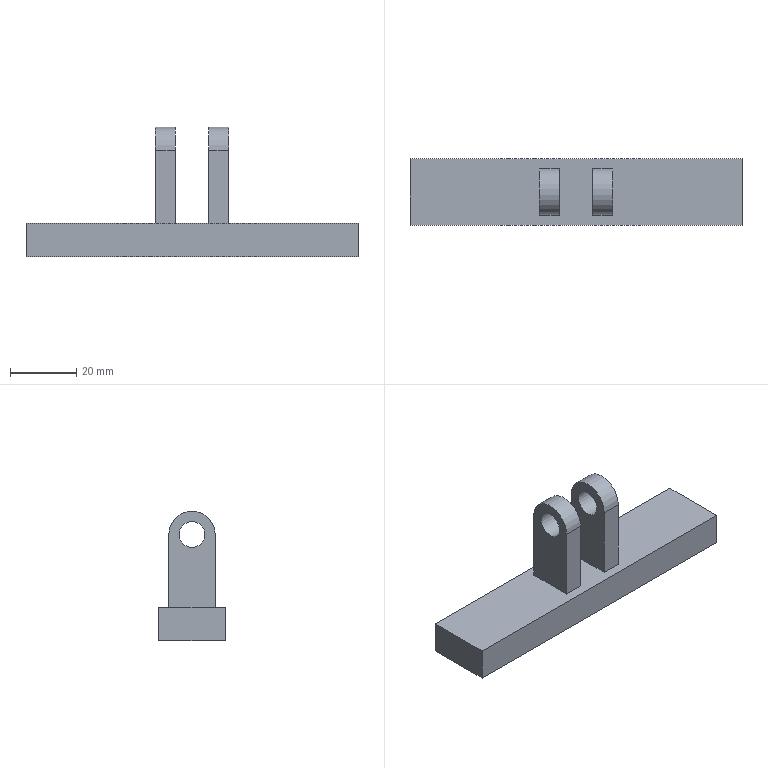Part | NX | features DATUM_CSYS 2, BLEND 1, BLOCK 1, EXTRUDE 1, HOLE PACKAGE 1, SIMPLE HOLE 1, SKETCH 1 | 1 solid | 18 faces | box 100 x 20 x 39 mm | volume 24046 mm3 | plane 14 | cylinder 4 | commonest cylinder face diameters 7.8 x2 14 x2
STEP:
#1=CARTESIAN_POINT('',(-11.,7.,10.));
#2=VERTEX_POINT('',#1);
#3=CARTESIAN_POINT('',(-11.,-7.,10.));
#4=VERTEX_POINT('',#3);
#5=CARTESIAN_POINT('',(-11.,7.,10.));
#6=DIRECTION('',(0.,-1.,0.));
#7=VECTOR('',#6,1000.);
#8=LINE('',#5,#7);
#9=EDGE_CURVE('',#2,#4,#8,.T.);
#10=ORIENTED_EDGE('',*,*,#9,.F.);
#11=CARTESIAN_POINT('',(-5.,7.,10.));
#12=VERTEX_POINT('',#11);
#13=CARTESIAN_POINT('',(-5.,7.,10.));
#14=DIRECTION('',(-1.,0.,0.));
#15=VECTOR('',#14,1000.);
#16=LINE('',#13,#15);
#17=EDGE_CURVE('',#12,#2,#16,.T.);
#18=ORIENTED_EDGE('',*,*,#17,.F.);
#19=CARTESIAN_POINT('',(-5.,-7.,10.));
#20=VERTEX_POINT('',#19);
#21=CARTESIAN_POINT('',(-5.,-7.,10.));
#22=DIRECTION('',(0.,1.,0.));
#23=VECTOR('',#22,1000.);
#24=LINE('',#21,#23);
#25=EDGE_CURVE('',#20,#12,#24,.T.);
#26=ORIENTED_EDGE('',*,*,#25,.F.);
#27=CARTESIAN_POINT('',(-11.,-7.,10.));
#28=DIRECTION('',(1.,0.,0.));
#29=VECTOR('',#28,1000.);
#30=LINE('',#27,#29);
#31=EDGE_CURVE('',#4,#20,#30,.T.);
#32=ORIENTED_EDGE('',*,*,#31,.F.);
#33=EDGE_LOOP('',(#10,#18,#26,#32));
#34=FACE_BOUND('',#33,.T.);
#35=CARTESIAN_POINT('',(5.,7.,10.));
#36=VERTEX_POINT('',#35);
#37=CARTESIAN_POINT('',(5.,-7.,10.));
#38=VERTEX_POINT('',#37);
#39=CARTESIAN_POINT('',(5.,7.,10.));
#40=DIRECTION('',(0.,-1.,0.));
#41=VECTOR('',#40,1000.);
#42=LINE('',#39,#41);
#43=EDGE_CURVE('',#36,#38,#42,.T.);
#44=ORIENTED_EDGE('',*,*,#43,.F.);
#45=CARTESIAN_POINT('',(11.,7.,10.));
#46=VERTEX_POINT('',#45);
#47=CARTESIAN_POINT('',(11.,7.,10.));
#48=DIRECTION('',(-1.,0.,0.));
#49=VECTOR('',#48,1000.);
#50=LINE('',#47,#49);
#51=EDGE_CURVE('',#46,#36,#50,.T.);
#52=ORIENTED_EDGE('',*,*,#51,.F.);
#53=CARTESIAN_POINT('',(11.,-7.,10.));
#54=VERTEX_POINT('',#53);
#55=CARTESIAN_POINT('',(11.,-7.,10.));
#56=DIRECTION('',(0.,1.,0.));
#57=VECTOR('',#56,1000.);
#58=LINE('',#55,#57);
#59=EDGE_CURVE('',#54,#46,#58,.T.);
#60=ORIENTED_EDGE('',*,*,#59,.F.);
#61=CARTESIAN_POINT('',(5.,-7.,10.));
#62=DIRECTION('',(1.,0.,0.));
#63=VECTOR('',#62,1000.);
#64=LINE('',#61,#63);
#65=EDGE_CURVE('',#38,#54,#64,.T.);
#66=ORIENTED_EDGE('',*,*,#65,.F.);
#67=EDGE_LOOP('',(#44,#52,#60,#66));
#68=FACE_BOUND('',#67,.T.);
#69=CARTESIAN_POINT('',(50.,-10.,10.));
#70=VERTEX_POINT('',#69);
#71=CARTESIAN_POINT('',(-50.,-10.,10.));
#72=VERTEX_POINT('',#71);
#73=CARTESIAN_POINT('',(0.,-10.,10.));
#74=DIRECTION('',(-1.,0.,0.));
#75=VECTOR('',#74,1000.);
#76=LINE('',#73,#75);
#77=EDGE_CURVE('',#70,#72,#76,.T.);
#78=ORIENTED_EDGE('',*,*,#77,.F.);
#79=CARTESIAN_POINT('',(50.,10.,10.));
#80=VERTEX_POINT('',#79);
#81=CARTESIAN_POINT('',(50.,0.,10.));
#82=DIRECTION('',(0.,-1.,0.));
#83=VECTOR('',#82,1000.);
#84=LINE('',#81,#83);
#85=EDGE_CURVE('',#80,#70,#84,.T.);
#86=ORIENTED_EDGE('',*,*,#85,.F.);
#87=CARTESIAN_POINT('',(-50.,10.,10.));
#88=VERTEX_POINT('',#87);
#89=CARTESIAN_POINT('',(0.,10.,10.));
#90=DIRECTION('',(1.,0.,0.));
#91=VECTOR('',#90,1000.);
#92=LINE('',#89,#91);
#93=EDGE_CURVE('',#88,#80,#92,.T.);
#94=ORIENTED_EDGE('',*,*,#93,.F.);
#95=CARTESIAN_POINT('',(-50.,0.,10.));
#96=DIRECTION('',(0.,1.,0.));
#97=VECTOR('',#96,1000.);
#98=LINE('',#95,#97);
#99=EDGE_CURVE('',#72,#88,#98,.T.);
#100=ORIENTED_EDGE('',*,*,#99,.F.);
#101=EDGE_LOOP('',(#78,#86,#94,#100));
#102=FACE_BOUND('',#101,.T.);
#103=CARTESIAN_POINT('',(0.,0.,10.));
#104=DIRECTION('',(0.,0.,1.));
#105=DIRECTION('',(1.,0.,0.));
#106=AXIS2_PLACEMENT_3D('',#103,#104,#105);
#107=PLANE('',#106);
#108=ADVANCED_FACE('',(#34,#68,#102),#107,.T.);
#109=CARTESIAN_POINT('',(50.,-10.,0.));
#110=VERTEX_POINT('',#109);
#111=CARTESIAN_POINT('',(50.,-10.,0.));
#112=DIRECTION('',(0.,0.,1.));
#113=VECTOR('',#112,1000.);
#114=LINE('',#111,#113);
#115=EDGE_CURVE('',#110,#70,#114,.T.);
#116=ORIENTED_EDGE('',*,*,#115,.T.);
#117=ORIENTED_EDGE('',*,*,#77,.T.);
#118=CARTESIAN_POINT('',(-50.,-10.,0.));
#119=VERTEX_POINT('',#118);
#120=CARTESIAN_POINT('',(-50.,-10.,0.));
#121=DIRECTION('',(0.,0.,1.));
#122=VECTOR('',#121,1000.);
#123=LINE('',#120,#122);
#124=EDGE_CURVE('',#119,#72,#123,.T.);
#125=ORIENTED_EDGE('',*,*,#124,.F.);
#126=CARTESIAN_POINT('',(0.,-10.,0.));
#127=DIRECTION('',(1.,0.,0.));
#128=VECTOR('',#127,1000.);
#129=LINE('',#126,#128);
#130=EDGE_CURVE('',#119,#110,#129,.T.);
#131=ORIENTED_EDGE('',*,*,#130,.T.);
#132=EDGE_LOOP('',(#116,#117,#125,#131));
#133=FACE_BOUND('',#132,.T.);
#134=CARTESIAN_POINT('',(0.,-10.,0.));
#135=DIRECTION('',(0.,-1.,0.));
#136=DIRECTION('',(0.,0.,-1.));
#137=AXIS2_PLACEMENT_3D('',#134,#135,#136);
#138=PLANE('',#137);
#139=ADVANCED_FACE('',(#133),#138,.T.);
#140=ORIENTED_EDGE('',*,*,#124,.T.);
#141=ORIENTED_EDGE('',*,*,#99,.T.);
#142=CARTESIAN_POINT('',(-50.,10.,0.));
#143=VERTEX_POINT('',#142);
#144=CARTESIAN_POINT('',(-50.,10.,0.));
#145=DIRECTION('',(0.,0.,1.));
#146=VECTOR('',#145,1000.);
#147=LINE('',#144,#146);
#148=EDGE_CURVE('',#143,#88,#147,.T.);
#149=ORIENTED_EDGE('',*,*,#148,.F.);
#150=CARTESIAN_POINT('',(-50.,0.,0.));
#151=DIRECTION('',(0.,-1.,0.));
#152=VECTOR('',#151,1000.);
#153=LINE('',#150,#152);
#154=EDGE_CURVE('',#143,#119,#153,.T.);
#155=ORIENTED_EDGE('',*,*,#154,.T.);
#156=EDGE_LOOP('',(#140,#141,#149,#155));
#157=FACE_BOUND('',#156,.T.);
#158=CARTESIAN_POINT('',(-50.,0.,0.));
#159=DIRECTION('',(-1.,0.,0.));
#160=DIRECTION('',(0.,0.,1.));
#161=AXIS2_PLACEMENT_3D('',#158,#159,#160);
#162=PLANE('',#161);
#163=ADVANCED_FACE('',(#157),#162,.T.);
#164=ORIENTED_EDGE('',*,*,#148,.T.);
#165=ORIENTED_EDGE('',*,*,#93,.T.);
#166=CARTESIAN_POINT('',(50.,10.,0.));
#167=VERTEX_POINT('',#166);
#168=CARTESIAN_POINT('',(50.,10.,0.));
#169=DIRECTION('',(0.,0.,1.));
#170=VECTOR('',#169,1000.);
#171=LINE('',#168,#170);
#172=EDGE_CURVE('',#167,#80,#171,.T.);
#173=ORIENTED_EDGE('',*,*,#172,.F.);
#174=CARTESIAN_POINT('',(0.,10.,0.));
#175=DIRECTION('',(-1.,0.,0.));
#176=VECTOR('',#175,1000.);
#177=LINE('',#174,#176);
#178=EDGE_CURVE('',#167,#143,#177,.T.);
#179=ORIENTED_EDGE('',*,*,#178,.T.);
#180=EDGE_LOOP('',(#164,#165,#173,#179));
#181=FACE_BOUND('',#180,.T.);
#182=CARTESIAN_POINT('',(0.,10.,0.));
#183=DIRECTION('',(0.,1.,0.));
#184=DIRECTION('',(0.,0.,1.));
#185=AXIS2_PLACEMENT_3D('',#182,#183,#184);
#186=PLANE('',#185);
#187=ADVANCED_FACE('',(#181),#186,.T.);
#188=CARTESIAN_POINT('',(50.,0.,0.));
#189=DIRECTION('',(0.,1.,0.));
#190=VECTOR('',#189,1000.);
#191=LINE('',#188,#190);
#192=EDGE_CURVE('',#110,#167,#191,.T.);
#193=ORIENTED_EDGE('',*,*,#192,.F.);
#194=ORIENTED_EDGE('',*,*,#130,.F.);
#195=ORIENTED_EDGE('',*,*,#154,.F.);
#196=ORIENTED_EDGE('',*,*,#178,.F.);
#197=EDGE_LOOP('',(#193,#194,#195,#196));
#198=FACE_BOUND('',#197,.T.);
#199=CARTESIAN_POINT('',(0.,0.,0.));
#200=DIRECTION('',(0.,0.,-1.));
#201=DIRECTION('',(-1.,0.,0.));
#202=AXIS2_PLACEMENT_3D('',#199,#200,#201);
#203=PLANE('',#202);
#204=ADVANCED_FACE('',(#198),#203,.T.);
#205=ORIENTED_EDGE('',*,*,#192,.T.);
#206=ORIENTED_EDGE('',*,*,#172,.T.);
#207=ORIENTED_EDGE('',*,*,#85,.T.);
#208=ORIENTED_EDGE('',*,*,#115,.F.);
#209=EDGE_LOOP('',(#205,#206,#207,#208));
#210=FACE_BOUND('',#209,.T.);
#211=CARTESIAN_POINT('',(50.,0.,0.));
#212=DIRECTION('',(1.,0.,0.));
#213=DIRECTION('',(0.,0.,-1.));
#214=AXIS2_PLACEMENT_3D('',#211,#212,#213);
#215=PLANE('',#214);
#216=ADVANCED_FACE('',(#210),#215,.T.);
#217=CARTESIAN_POINT('',(5.,3.9,32.));
#218=VERTEX_POINT('',#217);
#219=CARTESIAN_POINT('',(5.,0.,32.));
#220=DIRECTION('',(1.,0.,0.));
#221=DIRECTION('',(0.,1.,0.));
#222=AXIS2_PLACEMENT_3D('',#219,#220,#221);
#223=CIRCLE('',#222,3.9);
#224=EDGE_CURVE('',#218,#218,#223,.T.);
#225=ORIENTED_EDGE('',*,*,#224,.T.);
#226=EDGE_LOOP('',(#225));
#227=FACE_BOUND('',#226,.T.);
#228=CARTESIAN_POINT('',(5.,-7.,32.));
#229=VERTEX_POINT('',#228);
#230=CARTESIAN_POINT('',(5.,7.,32.));
#231=VERTEX_POINT('',#230);
#232=CARTESIAN_POINT('',(5.,0.,32.));
#233=DIRECTION('',(1.,0.,0.));
#234=DIRECTION('',(0.,1.,0.));
#235=AXIS2_PLACEMENT_3D('',#232,#233,#234);
#236=CIRCLE('',#235,7.);
#237=EDGE_CURVE('',#229,#231,#236,.F.);
#238=ORIENTED_EDGE('',*,*,#237,.T.);
#239=CARTESIAN_POINT('',(5.,7.,39.));
#240=DIRECTION('',(0.,0.,-1.));
#241=VECTOR('',#240,1000.);
#242=LINE('',#239,#241);
#243=EDGE_CURVE('',#231,#36,#242,.T.);
#244=ORIENTED_EDGE('',*,*,#243,.T.);
#245=ORIENTED_EDGE('',*,*,#43,.T.);
#246=CARTESIAN_POINT('',(5.,-7.,39.));
#247=DIRECTION('',(0.,0.,-1.));
#248=VECTOR('',#247,1000.);
#249=LINE('',#246,#248);
#250=EDGE_CURVE('',#229,#38,#249,.T.);
#251=ORIENTED_EDGE('',*,*,#250,.F.);
#252=EDGE_LOOP('',(#238,#244,#245,#251));
#253=FACE_BOUND('',#252,.T.);
#254=CARTESIAN_POINT('',(5.,7.,39.));
#255=DIRECTION('',(1.,0.,0.));
#256=DIRECTION('',(0.,1.,0.));
#257=AXIS2_PLACEMENT_3D('',#254,#255,#256);
#258=PLANE('',#257);
#259=ADVANCED_FACE('',(#227,#253),#258,.F.);
#260=CARTESIAN_POINT('',(11.,-7.,32.));
#261=VERTEX_POINT('',#260);
#262=CARTESIAN_POINT('',(11.,-7.,39.));
#263=DIRECTION('',(0.,0.,-1.));
#264=VECTOR('',#263,1000.);
#265=LINE('',#262,#264);
#266=EDGE_CURVE('',#261,#54,#265,.T.);
#267=ORIENTED_EDGE('',*,*,#266,.F.);
#268=CARTESIAN_POINT('',(5.,-7.,32.));
#269=DIRECTION('',(1.,0.,0.));
#270=VECTOR('',#269,1000.);
#271=LINE('',#268,#270);
#272=EDGE_CURVE('',#261,#229,#271,.F.);
#273=ORIENTED_EDGE('',*,*,#272,.T.);
#274=ORIENTED_EDGE('',*,*,#250,.T.);
#275=ORIENTED_EDGE('',*,*,#65,.T.);
#276=EDGE_LOOP('',(#267,#273,#274,#275));
#277=FACE_BOUND('',#276,.T.);
#278=CARTESIAN_POINT('',(5.,-7.,39.));
#279=DIRECTION('',(0.,1.,0.));
#280=DIRECTION('',(0.,0.,1.));
#281=AXIS2_PLACEMENT_3D('',#278,#279,#280);
#282=PLANE('',#281);
#283=ADVANCED_FACE('',(#277),#282,.F.);
#284=CARTESIAN_POINT('',(11.,-3.9,32.));
#285=VERTEX_POINT('',#284);
#286=CARTESIAN_POINT('',(11.,0.,32.));
#287=DIRECTION('',(-1.,0.,0.));
#288=DIRECTION('',(0.,-1.,0.));
#289=AXIS2_PLACEMENT_3D('',#286,#287,#288);
#290=CIRCLE('',#289,3.9);
#291=EDGE_CURVE('',#285,#285,#290,.T.);
#292=ORIENTED_EDGE('',*,*,#291,.T.);
#293=EDGE_LOOP('',(#292));
#294=FACE_BOUND('',#293,.T.);
#295=CARTESIAN_POINT('',(11.,7.,32.));
#296=VERTEX_POINT('',#295);
#297=CARTESIAN_POINT('',(11.,7.,39.));
#298=DIRECTION('',(0.,0.,-1.));
#299=VECTOR('',#298,1000.);
#300=LINE('',#297,#299);
#301=EDGE_CURVE('',#296,#46,#300,.T.);
#302=ORIENTED_EDGE('',*,*,#301,.F.);
#303=CARTESIAN_POINT('',(11.,0.,32.));
#304=DIRECTION('',(-1.,0.,0.));
#305=DIRECTION('',(0.,-1.,0.));
#306=AXIS2_PLACEMENT_3D('',#303,#304,#305);
#307=CIRCLE('',#306,7.);
#308=EDGE_CURVE('',#296,#261,#307,.F.);
#309=ORIENTED_EDGE('',*,*,#308,.T.);
#310=ORIENTED_EDGE('',*,*,#266,.T.);
#311=ORIENTED_EDGE('',*,*,#59,.T.);
#312=EDGE_LOOP('',(#302,#309,#310,#311));
#313=FACE_BOUND('',#312,.T.);
#314=CARTESIAN_POINT('',(11.,-7.,39.));
#315=DIRECTION('',(-1.,0.,0.));
#316=DIRECTION('',(0.,-1.,0.));
#317=AXIS2_PLACEMENT_3D('',#314,#315,#316);
#318=PLANE('',#317);
#319=ADVANCED_FACE('',(#294,#313),#318,.F.);
#320=ORIENTED_EDGE('',*,*,#243,.F.);
#321=CARTESIAN_POINT('',(11.,7.,32.));
#322=DIRECTION('',(-1.,0.,0.));
#323=VECTOR('',#322,1000.);
#324=LINE('',#321,#323);
#325=EDGE_CURVE('',#231,#296,#324,.F.);
#326=ORIENTED_EDGE('',*,*,#325,.T.);
#327=ORIENTED_EDGE('',*,*,#301,.T.);
#328=ORIENTED_EDGE('',*,*,#51,.T.);
#329=EDGE_LOOP('',(#320,#326,#327,#328));
#330=FACE_BOUND('',#329,.T.);
#331=CARTESIAN_POINT('',(11.,7.,39.));
#332=DIRECTION('',(0.,-1.,0.));
#333=DIRECTION('',(1.,0.,0.));
#334=AXIS2_PLACEMENT_3D('',#331,#332,#333);
#335=PLANE('',#334);
#336=ADVANCED_FACE('',(#330),#335,.F.);
#337=CARTESIAN_POINT('',(-11.,3.9,32.));
#338=VERTEX_POINT('',#337);
#339=CARTESIAN_POINT('',(-11.,0.,32.));
#340=DIRECTION('',(1.,0.,0.));
#341=DIRECTION('',(0.,1.,0.));
#342=AXIS2_PLACEMENT_3D('',#339,#340,#341);
#343=CIRCLE('',#342,3.9);
#344=EDGE_CURVE('',#338,#338,#343,.T.);
#345=ORIENTED_EDGE('',*,*,#344,.T.);
#346=EDGE_LOOP('',(#345));
#347=FACE_BOUND('',#346,.T.);
#348=CARTESIAN_POINT('',(-11.,-7.,32.));
#349=VERTEX_POINT('',#348);
#350=CARTESIAN_POINT('',(-11.,7.,32.));
#351=VERTEX_POINT('',#350);
#352=CARTESIAN_POINT('',(-11.,0.,32.));
#353=DIRECTION('',(1.,0.,0.));
#354=DIRECTION('',(0.,1.,0.));
#355=AXIS2_PLACEMENT_3D('',#352,#353,#354);
#356=CIRCLE('',#355,7.);
#357=EDGE_CURVE('',#349,#351,#356,.F.);
#358=ORIENTED_EDGE('',*,*,#357,.T.);
#359=CARTESIAN_POINT('',(-11.,7.,39.));
#360=DIRECTION('',(0.,0.,-1.));
#361=VECTOR('',#360,1000.);
#362=LINE('',#359,#361);
#363=EDGE_CURVE('',#351,#2,#362,.T.);
#364=ORIENTED_EDGE('',*,*,#363,.T.);
#365=ORIENTED_EDGE('',*,*,#9,.T.);
#366=CARTESIAN_POINT('',(-11.,-7.,39.));
#367=DIRECTION('',(0.,0.,-1.));
#368=VECTOR('',#367,1000.);
#369=LINE('',#366,#368);
#370=EDGE_CURVE('',#349,#4,#369,.T.);
#371=ORIENTED_EDGE('',*,*,#370,.F.);
#372=EDGE_LOOP('',(#358,#364,#365,#371));
#373=FACE_BOUND('',#372,.T.);
#374=CARTESIAN_POINT('',(-11.,7.,39.));
#375=DIRECTION('',(1.,0.,0.));
#376=DIRECTION('',(0.,1.,0.));
#377=AXIS2_PLACEMENT_3D('',#374,#375,#376);
#378=PLANE('',#377);
#379=ADVANCED_FACE('',(#347,#373),#378,.F.);
#380=CARTESIAN_POINT('',(-5.,-7.,32.));
#381=VERTEX_POINT('',#380);
#382=CARTESIAN_POINT('',(-5.,-7.,39.));
#383=DIRECTION('',(0.,0.,-1.));
#384=VECTOR('',#383,1000.);
#385=LINE('',#382,#384);
#386=EDGE_CURVE('',#381,#20,#385,.T.);
#387=ORIENTED_EDGE('',*,*,#386,.F.);
#388=CARTESIAN_POINT('',(-11.,-7.,32.));
#389=DIRECTION('',(1.,0.,0.));
#390=VECTOR('',#389,1000.);
#391=LINE('',#388,#390);
#392=EDGE_CURVE('',#381,#349,#391,.F.);
#393=ORIENTED_EDGE('',*,*,#392,.T.);
#394=ORIENTED_EDGE('',*,*,#370,.T.);
#395=ORIENTED_EDGE('',*,*,#31,.T.);
#396=EDGE_LOOP('',(#387,#393,#394,#395));
#397=FACE_BOUND('',#396,.T.);
#398=CARTESIAN_POINT('',(-11.,-7.,39.));
#399=DIRECTION('',(0.,1.,0.));
#400=DIRECTION('',(0.,0.,1.));
#401=AXIS2_PLACEMENT_3D('',#398,#399,#400);
#402=PLANE('',#401);
#403=ADVANCED_FACE('',(#397),#402,.F.);
#404=CARTESIAN_POINT('',(-5.,-3.9,32.));
#405=VERTEX_POINT('',#404);
#406=CARTESIAN_POINT('',(-5.,0.,32.));
#407=DIRECTION('',(-1.,0.,0.));
#408=DIRECTION('',(0.,-1.,0.));
#409=AXIS2_PLACEMENT_3D('',#406,#407,#408);
#410=CIRCLE('',#409,3.9);
#411=EDGE_CURVE('',#405,#405,#410,.T.);
#412=ORIENTED_EDGE('',*,*,#411,.T.);
#413=EDGE_LOOP('',(#412));
#414=FACE_BOUND('',#413,.T.);
#415=CARTESIAN_POINT('',(-5.,7.,32.));
#416=VERTEX_POINT('',#415);
#417=CARTESIAN_POINT('',(-5.,7.,39.));
#418=DIRECTION('',(0.,0.,-1.));
#419=VECTOR('',#418,1000.);
#420=LINE('',#417,#419);
#421=EDGE_CURVE('',#416,#12,#420,.T.);
#422=ORIENTED_EDGE('',*,*,#421,.F.);
#423=CARTESIAN_POINT('',(-5.,0.,32.));
#424=DIRECTION('',(-1.,0.,0.));
#425=DIRECTION('',(0.,-1.,0.));
#426=AXIS2_PLACEMENT_3D('',#423,#424,#425);
#427=CIRCLE('',#426,7.);
#428=EDGE_CURVE('',#416,#381,#427,.F.);
#429=ORIENTED_EDGE('',*,*,#428,.T.);
#430=ORIENTED_EDGE('',*,*,#386,.T.);
#431=ORIENTED_EDGE('',*,*,#25,.T.);
#432=EDGE_LOOP('',(#422,#429,#430,#431));
#433=FACE_BOUND('',#432,.T.);
#434=CARTESIAN_POINT('',(-5.,-7.,39.));
#435=DIRECTION('',(-1.,0.,0.));
#436=DIRECTION('',(0.,-1.,0.));
#437=AXIS2_PLACEMENT_3D('',#434,#435,#436);
#438=PLANE('',#437);
#439=ADVANCED_FACE('',(#414,#433),#438,.F.);
#440=ORIENTED_EDGE('',*,*,#363,.F.);
#441=CARTESIAN_POINT('',(-5.,7.,32.));
#442=DIRECTION('',(-1.,0.,0.));
#443=VECTOR('',#442,1000.);
#444=LINE('',#441,#443);
#445=EDGE_CURVE('',#351,#416,#444,.F.);
#446=ORIENTED_EDGE('',*,*,#445,.T.);
#447=ORIENTED_EDGE('',*,*,#421,.T.);
#448=ORIENTED_EDGE('',*,*,#17,.T.);
#449=EDGE_LOOP('',(#440,#446,#447,#448));
#450=FACE_BOUND('',#449,.T.);
#451=CARTESIAN_POINT('',(-5.,7.,39.));
#452=DIRECTION('',(0.,-1.,0.));
#453=DIRECTION('',(1.,0.,0.));
#454=AXIS2_PLACEMENT_3D('',#451,#452,#453);
#455=PLANE('',#454);
#456=ADVANCED_FACE('',(#450),#455,.F.);
#457=ORIENTED_EDGE('',*,*,#392,.F.);
#458=ORIENTED_EDGE('',*,*,#428,.F.);
#459=ORIENTED_EDGE('',*,*,#445,.F.);
#460=ORIENTED_EDGE('',*,*,#357,.F.);
#461=EDGE_LOOP('',(#457,#458,#459,#460));
#462=FACE_BOUND('',#461,.T.);
#463=CARTESIAN_POINT('',(0.,0.,32.));
#464=DIRECTION('',(-1.,0.,0.));
#465=DIRECTION('',(0.,0.,1.));
#466=AXIS2_PLACEMENT_3D('',#463,#464,#465);
#467=CYLINDRICAL_SURFACE('',#466,7.);
#468=ADVANCED_FACE('',(#462),#467,.T.);
#469=ORIENTED_EDGE('',*,*,#272,.F.);
#470=ORIENTED_EDGE('',*,*,#308,.F.);
#471=ORIENTED_EDGE('',*,*,#325,.F.);
#472=ORIENTED_EDGE('',*,*,#237,.F.);
#473=EDGE_LOOP('',(#469,#470,#471,#472));
#474=FACE_BOUND('',#473,.T.);
#475=CARTESIAN_POINT('',(0.,0.,32.));
#476=DIRECTION('',(-1.,0.,0.));
#477=DIRECTION('',(0.,0.,1.));
#478=AXIS2_PLACEMENT_3D('',#475,#476,#477);
#479=CYLINDRICAL_SURFACE('',#478,7.);
#480=ADVANCED_FACE('',(#474),#479,.T.);
#481=ORIENTED_EDGE('',*,*,#411,.F.);
#482=EDGE_LOOP('',(#481));
#483=FACE_BOUND('',#482,.T.);
#484=ORIENTED_EDGE('',*,*,#344,.F.);
#485=EDGE_LOOP('',(#484));
#486=FACE_BOUND('',#485,.T.);
#487=CARTESIAN_POINT('',(11.,0.,32.));
#488=DIRECTION('',(-1.,0.,0.));
#489=DIRECTION('',(0.,-1.,0.));
#490=AXIS2_PLACEMENT_3D('',#487,#488,#489);
#491=CYLINDRICAL_SURFACE('',#490,3.9);
#492=ADVANCED_FACE('',(#483,#486),#491,.F.);
#493=ORIENTED_EDGE('',*,*,#291,.F.);
#494=EDGE_LOOP('',(#493));
#495=FACE_BOUND('',#494,.T.);
#496=ORIENTED_EDGE('',*,*,#224,.F.);
#497=EDGE_LOOP('',(#496));
#498=FACE_BOUND('',#497,.T.);
#499=CARTESIAN_POINT('',(11.,0.,32.));
#500=DIRECTION('',(-1.,0.,0.));
#501=DIRECTION('',(0.,-1.,0.));
#502=AXIS2_PLACEMENT_3D('',#499,#500,#501);
#503=CYLINDRICAL_SURFACE('',#502,3.9);
#504=ADVANCED_FACE('',(#495,#498),#503,.F.);
#505=CLOSED_SHELL('',(#108,#139,#163,#187,#204,#216,#259,#283,#319,#336,#379,#403,#439,#456,#468,#480,#492,#504));
#506=MANIFOLD_SOLID_BREP('',#505);
#507=(LENGTH_UNIT()NAMED_UNIT(*)SI_UNIT(.MILLI.,.METRE.));
#508=UNCERTAINTY_MEASURE_WITH_UNIT(LENGTH_MEASURE(0.00001),#507,'','');
#509=(NAMED_UNIT(*)PLANE_ANGLE_UNIT()SI_UNIT($,.RADIAN.));
#510=(NAMED_UNIT(*)SI_UNIT($,.STERADIAN.)SOLID_ANGLE_UNIT());
#511=(GEOMETRIC_REPRESENTATION_CONTEXT(3)GLOBAL_UNCERTAINTY_ASSIGNED_CONTEXT((#508))GLOBAL_UNIT_ASSIGNED_CONTEXT((#507,#509,#510))REPRESENTATION_CONTEXT('',''));
#512=ADVANCED_BREP_SHAPE_REPRESENTATION('',(#506),#511);